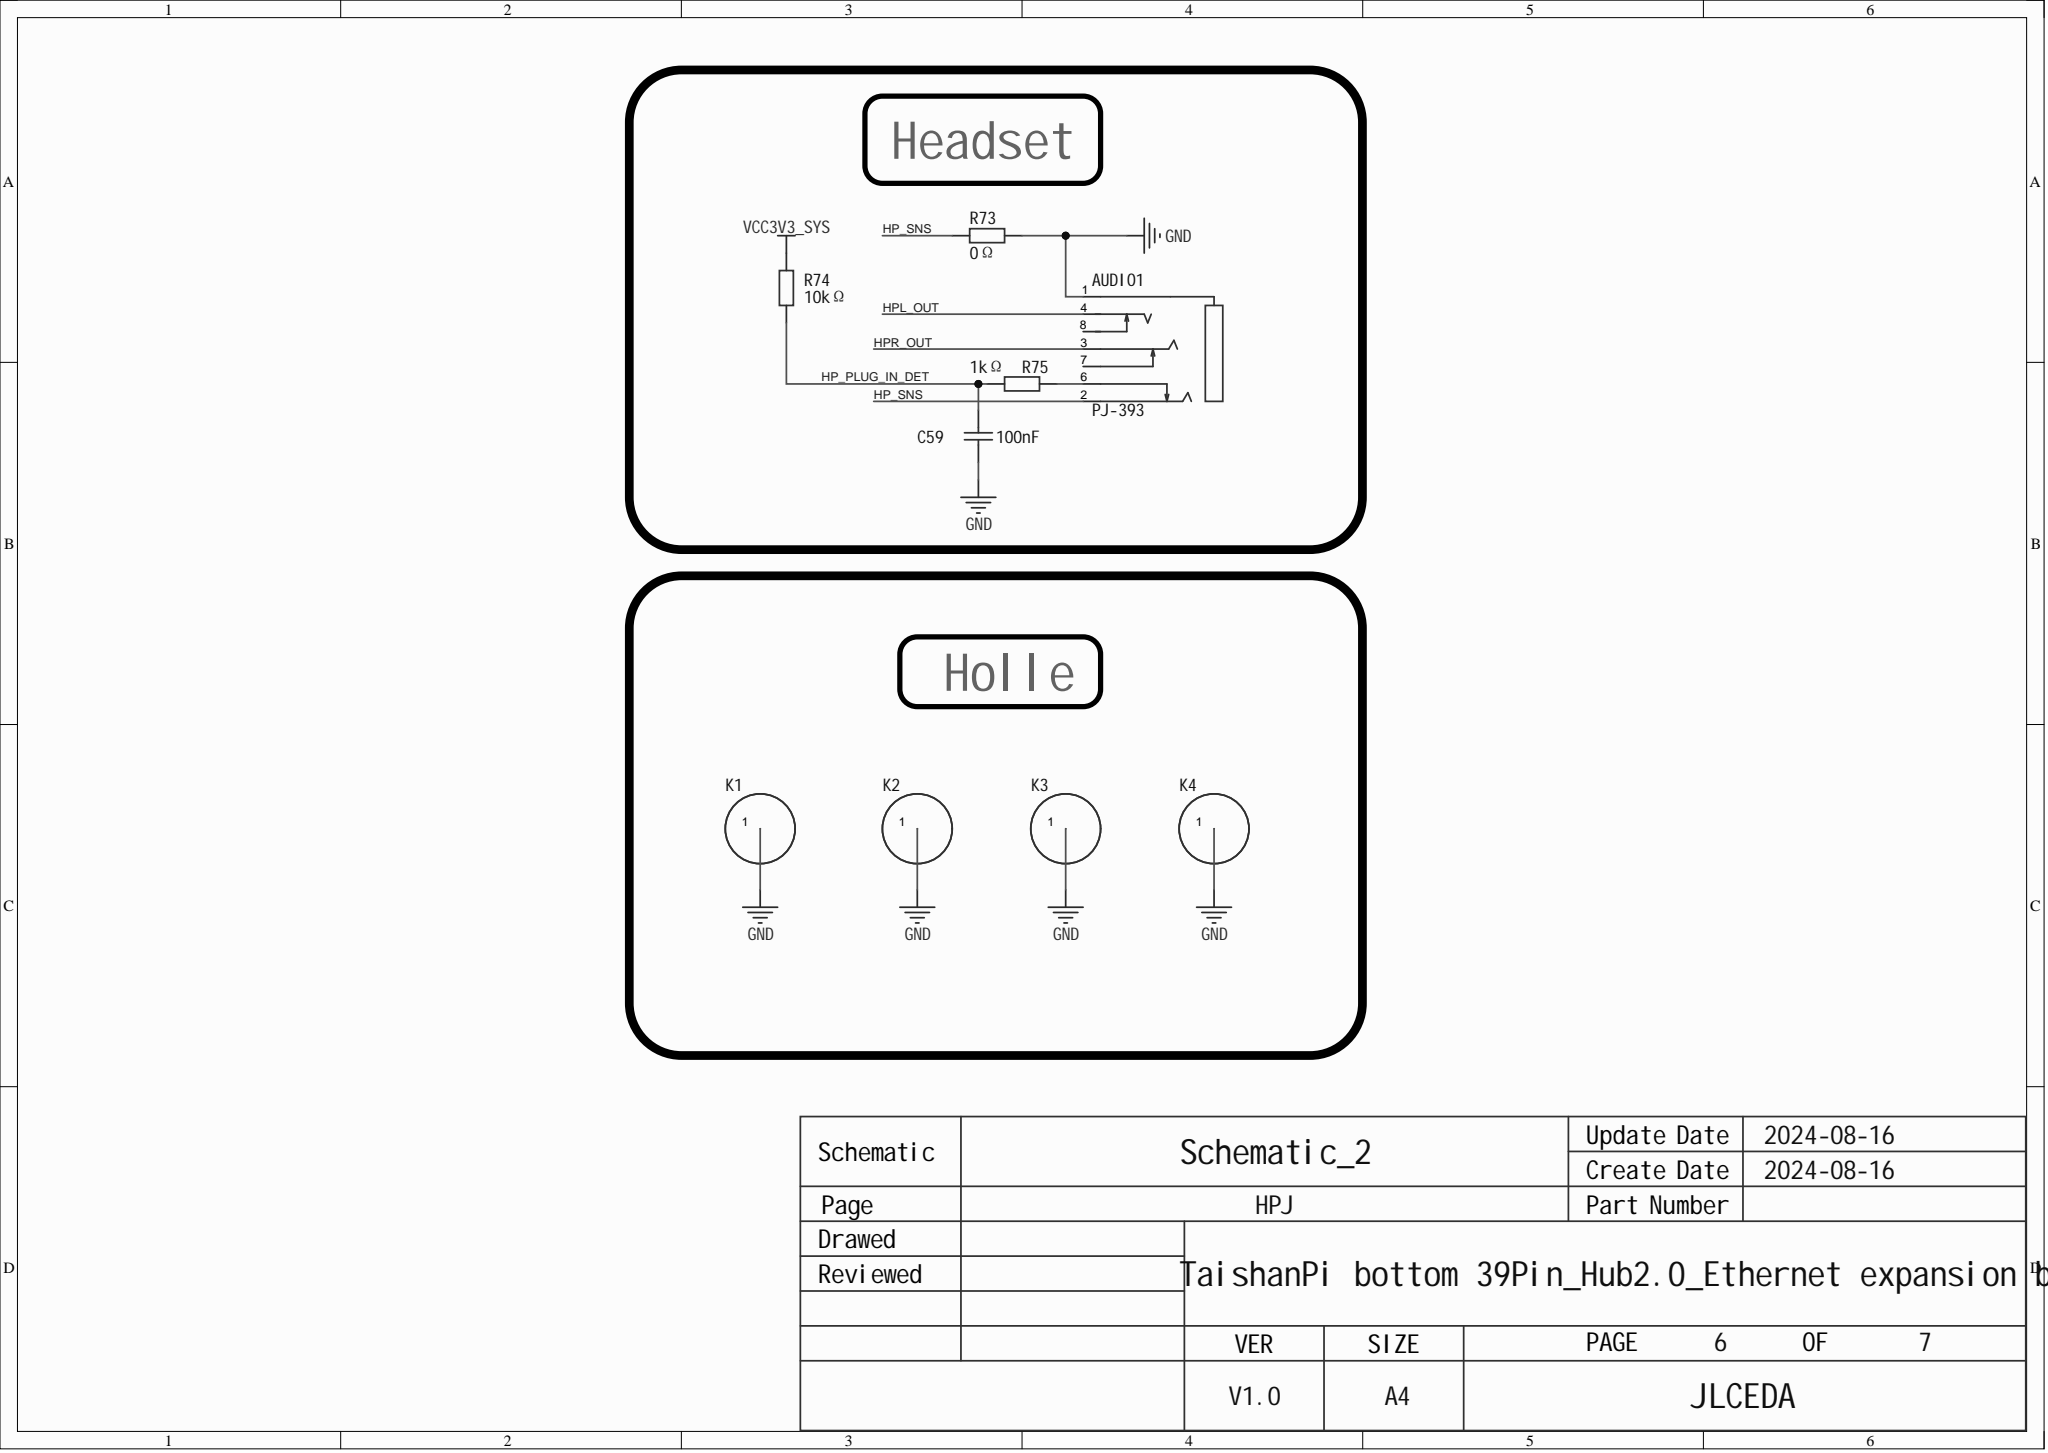Circuit board | Altium Designer | 209 parts | 149 nets | one sheet of the schematic
Parts on this sheet (reference | value | footprint):
AUDIO1 | PJ-393 | AUDIO-SMD_PJ-393
C59 | 100nF | R0402
K1 | 125 X 300
K2 | 125 X 300
K3 | 125 X 300
K4 | 125 X 300
R73 | 0Ω | R0402
R74 | 10kΩ | R0402
R75 | 1kΩ | R0402
Nets of these parts (net: part-pin ...):
VCC3V3_SYS: R74-2
NetAUDIO1_6: AUDIO1-6 R75-2
HPR_OUT: AUDIO1-3
HPL_OUT: AUDIO1-4
HP_SNS: AUDIO1-2 R73-1
GPIO0_C5: C59-1 R74-1 R75-1
GND: AUDIO1-1 C59-2 K1-1 K2-1 K3-1 K4-1 R73-2